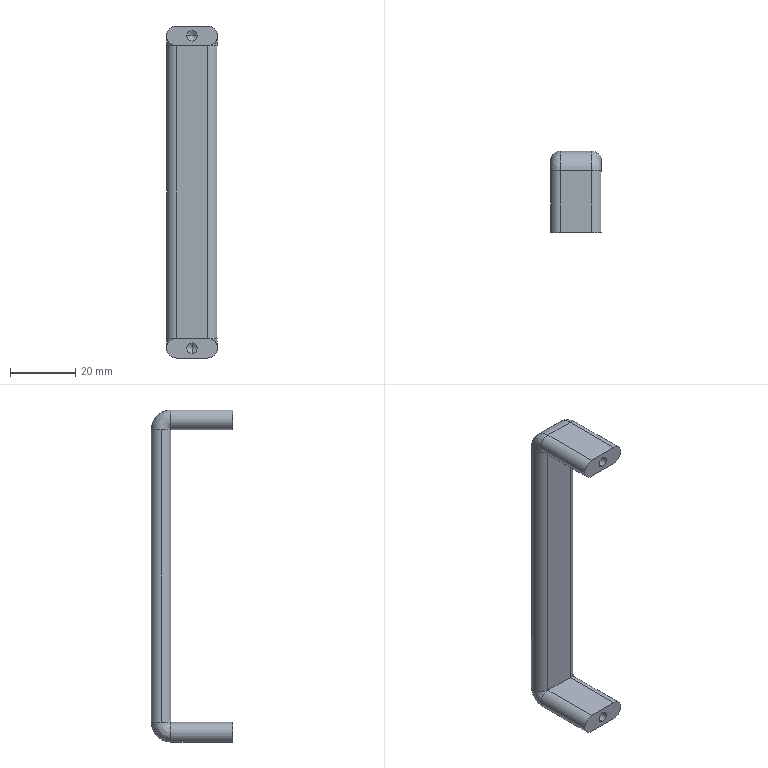Part | STEP file | AKM01-96 handle | 1 solid | 29 faces | box 15.6 x 25 x 102 mm | volume 11694 mm3 | cylinder 13 | plane 8 | cone 4 | spline 4 | commonest cylinder face diameters 6 x7 3.242 x4 12 x2
STEP:
#1=CARTESIAN_POINT('',(-4.8,19.,-6.));
#2=VERTEX_POINT('',#1);
#3=CARTESIAN_POINT('',(-7.8,22.,-6.));
#4=VERTEX_POINT('',#3);
#5=CARTESIAN_POINT('',(-4.8,22.,-6.));
#6=DIRECTION('',(0.,0.,-1.));
#7=DIRECTION('',(-1.,0.,0.));
#8=AXIS2_PLACEMENT_3D('',#5,#6,#7);
#9=CIRCLE('',#8,3.);
#10=EDGE_CURVE('',#2,#4,#9,.T.);
#11=ORIENTED_EDGE('',*,*,#10,.T.);
#12=CARTESIAN_POINT('',(-7.8,22.,-96.));
#13=VERTEX_POINT('',#12);
#14=CARTESIAN_POINT('',(-7.8,22.,-96.));
#15=DIRECTION('',(0.,0.,-1.));
#16=VECTOR('',#15,1000.);
#17=LINE('',#14,#16);
#18=EDGE_CURVE('',#4,#13,#17,.T.);
#19=ORIENTED_EDGE('',*,*,#18,.T.);
#20=CARTESIAN_POINT('',(-4.8,19.,-96.));
#21=VERTEX_POINT('',#20);
#22=CARTESIAN_POINT('',(-4.8,22.,-96.));
#23=DIRECTION('',(0.,0.,1.));
#24=DIRECTION('',(-1.,0.,0.));
#25=AXIS2_PLACEMENT_3D('',#22,#23,#24);
#26=CIRCLE('',#25,3.);
#27=EDGE_CURVE('',#13,#21,#26,.T.);
#28=ORIENTED_EDGE('',*,*,#27,.T.);
#29=CARTESIAN_POINT('',(-4.8,19.,-96.));
#30=DIRECTION('',(0.,0.,1.));
#31=VECTOR('',#30,1000.);
#32=LINE('',#29,#31);
#33=EDGE_CURVE('',#21,#2,#32,.T.);
#34=ORIENTED_EDGE('',*,*,#33,.T.);
#35=EDGE_LOOP('',(#11,#19,#28,#34));
#36=FACE_OUTER_BOUND('',#35,.T.);
#37=CARTESIAN_POINT('',(-4.8,22.,-96.));
#38=DIRECTION('',(0.,0.,-1.));
#39=DIRECTION('',(-1.,0.,0.));
#40=AXIS2_PLACEMENT_3D('',#37,#38,#39);
#41=CYLINDRICAL_SURFACE('',#40,3.);
#42=ADVANCED_FACE('',(#36),#41,.T.);
#43=CARTESIAN_POINT('',(0.,0.,-100.621));
#44=VERTEX_POINT('',#43);
#45=CARTESIAN_POINT('',(0.,0.,-97.379));
#46=VERTEX_POINT('',#45);
#47=CARTESIAN_POINT('',(0.,0.,-99.));
#48=DIRECTION('',(0.,1.,0.));
#49=DIRECTION('',(0.,0.,1.));
#50=AXIS2_PLACEMENT_3D('',#47,#48,#49);
#51=CIRCLE('',#50,1.621);
#52=EDGE_CURVE('',#44,#46,#51,.T.);
#53=ORIENTED_EDGE('',*,*,#52,.F.);
#54=CARTESIAN_POINT('',(0.,6.219,-100.621));
#55=VERTEX_POINT('',#54);
#56=CARTESIAN_POINT('',(0.,0.,-100.621));
#57=DIRECTION('',(0.,1.,0.));
#58=VECTOR('',#57,1000.);
#59=LINE('',#56,#58);
#60=EDGE_CURVE('',#44,#55,#59,.T.);
#61=ORIENTED_EDGE('',*,*,#60,.T.);
#62=CARTESIAN_POINT('',(0.,6.219,-97.379));
#63=VERTEX_POINT('',#62);
#64=CARTESIAN_POINT('',(0.,6.219,-99.));
#65=DIRECTION('',(0.,-1.,0.));
#66=DIRECTION('',(0.,0.,1.));
#67=AXIS2_PLACEMENT_3D('',#64,#65,#66);
#68=CIRCLE('',#67,1.621);
#69=EDGE_CURVE('',#63,#55,#68,.T.);
#70=ORIENTED_EDGE('',*,*,#69,.F.);
#71=CARTESIAN_POINT('',(0.,0.,-97.379));
#72=DIRECTION('',(0.,1.,0.));
#73=VECTOR('',#72,1000.);
#74=LINE('',#71,#73);
#75=EDGE_CURVE('',#46,#63,#74,.T.);
#76=ORIENTED_EDGE('',*,*,#75,.F.);
#77=EDGE_LOOP('',(#53,#61,#70,#76));
#78=FACE_OUTER_BOUND('',#77,.T.);
#79=CARTESIAN_POINT('',(0.,0.,-99.));
#80=DIRECTION('',(0.,1.,0.));
#81=DIRECTION('',(0.,0.,1.));
#82=AXIS2_PLACEMENT_3D('',#79,#80,#81);
#83=CYLINDRICAL_SURFACE('',#82,1.621);
#84=ADVANCED_FACE('',(#78),#83,.F.);
#85=CARTESIAN_POINT('',(0.,0.,-1.379));
#86=VERTEX_POINT('',#85);
#87=CARTESIAN_POINT('',(0.,0.,-4.621));
#88=VERTEX_POINT('',#87);
#89=CARTESIAN_POINT('',(0.,0.,-3.));
#90=DIRECTION('',(0.,-1.,0.));
#91=DIRECTION('',(0.,0.,1.));
#92=AXIS2_PLACEMENT_3D('',#89,#90,#91);
#93=CIRCLE('',#92,1.621);
#94=EDGE_CURVE('',#86,#88,#93,.T.);
#95=ORIENTED_EDGE('',*,*,#94,.T.);
#96=CARTESIAN_POINT('',(0.,6.219,-4.621));
#97=VERTEX_POINT('',#96);
#98=CARTESIAN_POINT('',(0.,0.,-4.621));
#99=DIRECTION('',(0.,1.,0.));
#100=VECTOR('',#99,1000.);
#101=LINE('',#98,#100);
#102=EDGE_CURVE('',#88,#97,#101,.T.);
#103=ORIENTED_EDGE('',*,*,#102,.T.);
#104=CARTESIAN_POINT('',(-1.621,6.219,-3.));
#105=VERTEX_POINT('',#104);
#106=CARTESIAN_POINT('',(0.,6.219,-3.));
#107=DIRECTION('',(0.,-1.,0.));
#108=DIRECTION('',(0.,0.,1.));
#109=AXIS2_PLACEMENT_3D('',#106,#107,#108);
#110=CIRCLE('',#109,1.621);
#111=EDGE_CURVE('',#105,#97,#110,.T.);
#112=ORIENTED_EDGE('',*,*,#111,.F.);
#113=CARTESIAN_POINT('',(0.,6.219,-1.379));
#114=VERTEX_POINT('',#113);
#115=CARTESIAN_POINT('',(0.,6.219,-3.));
#116=DIRECTION('',(0.,-1.,0.));
#117=DIRECTION('',(0.,0.,1.));
#118=AXIS2_PLACEMENT_3D('',#115,#116,#117);
#119=CIRCLE('',#118,1.621);
#120=EDGE_CURVE('',#114,#105,#119,.T.);
#121=ORIENTED_EDGE('',*,*,#120,.F.);
#122=CARTESIAN_POINT('',(0.,0.,-1.379));
#123=DIRECTION('',(0.,1.,0.));
#124=VECTOR('',#123,1000.);
#125=LINE('',#122,#124);
#126=EDGE_CURVE('',#86,#114,#125,.T.);
#127=ORIENTED_EDGE('',*,*,#126,.F.);
#128=EDGE_LOOP('',(#95,#103,#112,#121,#127));
#129=FACE_OUTER_BOUND('',#128,.T.);
#130=CARTESIAN_POINT('',(0.,0.,-3.));
#131=DIRECTION('',(0.,1.,0.));
#132=DIRECTION('',(0.,0.,1.));
#133=AXIS2_PLACEMENT_3D('',#130,#131,#132);
#134=CYLINDRICAL_SURFACE('',#133,1.621);
#135=ADVANCED_FACE('',(#129),#134,.F.);
#136=CARTESIAN_POINT('',(0.,7.155,-99.));
#137=VERTEX_POINT('',#136);
#138=CARTESIAN_POINT('',(0.,6.219,-100.621));
#139=DIRECTION('',(0.,-0.5,-0.866));
#140=VECTOR('',#139,1000.);
#141=LINE('',#138,#140);
#142=EDGE_CURVE('',#137,#55,#141,.T.);
#143=ORIENTED_EDGE('',*,*,#142,.F.);
#144=CARTESIAN_POINT('',(0.,6.219,-97.379));
#145=DIRECTION('',(0.,-0.5,0.866));
#146=VECTOR('',#145,1000.);
#147=LINE('',#144,#146);
#148=EDGE_CURVE('',#137,#63,#147,.T.);
#149=ORIENTED_EDGE('',*,*,#148,.T.);
#150=ORIENTED_EDGE('',*,*,#69,.T.);
#151=EDGE_LOOP('',(#143,#149,#150));
#152=FACE_OUTER_BOUND('',#151,.T.);
#153=CARTESIAN_POINT('',(0.,6.219,-99.));
#154=DIRECTION('',(0.,-1.,0.));
#155=DIRECTION('',(0.,0.,-1.));
#156=AXIS2_PLACEMENT_3D('',#153,#154,#155);
#157=CONICAL_SURFACE('',#156,1.621,1.047);
#158=ADVANCED_FACE('',(#152),#157,.F.);
#159=CARTESIAN_POINT('',(0.,7.155,-3.));
#160=VERTEX_POINT('',#159);
#161=CARTESIAN_POINT('',(1.621,6.219,-3.));
#162=VERTEX_POINT('',#161);
#163=CARTESIAN_POINT('',(1.621,6.219,-3.));
#164=DIRECTION('',(0.866,-0.5,0.));
#165=VECTOR('',#164,1000.);
#166=LINE('',#163,#165);
#167=EDGE_CURVE('',#160,#162,#166,.T.);
#168=ORIENTED_EDGE('',*,*,#167,.F.);
#169=CARTESIAN_POINT('',(-1.621,6.219,-3.));
#170=DIRECTION('',(-0.866,-0.5,0.));
#171=VECTOR('',#170,1000.);
#172=LINE('',#169,#171);
#173=EDGE_CURVE('',#160,#105,#172,.T.);
#174=ORIENTED_EDGE('',*,*,#173,.T.);
#175=ORIENTED_EDGE('',*,*,#111,.T.);
#176=CARTESIAN_POINT('',(0.,6.219,-3.));
#177=DIRECTION('',(0.,-1.,0.));
#178=DIRECTION('',(0.,0.,1.));
#179=AXIS2_PLACEMENT_3D('',#176,#177,#178);
#180=CIRCLE('',#179,1.621);
#181=EDGE_CURVE('',#97,#162,#180,.T.);
#182=ORIENTED_EDGE('',*,*,#181,.T.);
#183=EDGE_LOOP('',(#168,#174,#175,#182));
#184=FACE_OUTER_BOUND('',#183,.T.);
#185=CARTESIAN_POINT('',(0.,6.219,-3.));
#186=DIRECTION('',(0.,-1.,0.));
#187=DIRECTION('',(1.,0.,0.));
#188=AXIS2_PLACEMENT_3D('',#185,#186,#187);
#189=CONICAL_SURFACE('',#188,1.621,1.047);
#190=ADVANCED_FACE('',(#184),#189,.F.);
#191=CARTESIAN_POINT('',(4.8,19.,-6.));
#192=VERTEX_POINT('',#191);
#193=CARTESIAN_POINT('',(4.8,19.,-96.));
#194=VERTEX_POINT('',#193);
#195=CARTESIAN_POINT('',(4.8,19.,-96.));
#196=DIRECTION('',(0.,0.,-1.));
#197=VECTOR('',#196,1000.);
#198=LINE('',#195,#197);
#199=EDGE_CURVE('',#192,#194,#198,.T.);
#200=ORIENTED_EDGE('',*,*,#199,.F.);
#201=CARTESIAN_POINT('',(4.8,19.,-6.));
#202=DIRECTION('',(1.,0.,0.));
#203=VECTOR('',#202,1000.);
#204=LINE('',#201,#203);
#205=EDGE_CURVE('',#2,#192,#204,.T.);
#206=ORIENTED_EDGE('',*,*,#205,.F.);
#207=ORIENTED_EDGE('',*,*,#33,.F.);
#208=CARTESIAN_POINT('',(4.8,19.,-96.));
#209=DIRECTION('',(-1.,0.,0.));
#210=VECTOR('',#209,1000.);
#211=LINE('',#208,#210);
#212=EDGE_CURVE('',#194,#21,#211,.T.);
#213=ORIENTED_EDGE('',*,*,#212,.F.);
#214=EDGE_LOOP('',(#200,#206,#207,#213));
#215=FACE_OUTER_BOUND('',#214,.T.);
#216=CARTESIAN_POINT('',(4.8,19.,-96.));
#217=DIRECTION('',(0.,1.,0.));
#218=DIRECTION('',(0.,0.,1.));
#219=AXIS2_PLACEMENT_3D('',#216,#217,#218);
#220=PLANE('',#219);
#221=ADVANCED_FACE('',(#215),#220,.F.);
#222=CARTESIAN_POINT('',(-4.8,0.,-96.));
#223=VERTEX_POINT('',#222);
#224=CARTESIAN_POINT('',(-4.8,0.,-96.));
#225=DIRECTION('',(0.,1.,0.));
#226=VECTOR('',#225,1000.);
#227=LINE('',#224,#226);
#228=EDGE_CURVE('',#223,#21,#227,.T.);
#229=ORIENTED_EDGE('',*,*,#228,.F.);
#230=CARTESIAN_POINT('',(4.8,0.,-96.));
#231=VERTEX_POINT('',#230);
#232=CARTESIAN_POINT('',(4.8,0.,-96.));
#233=DIRECTION('',(-1.,0.,0.));
#234=VECTOR('',#233,1000.);
#235=LINE('',#232,#234);
#236=EDGE_CURVE('',#231,#223,#235,.T.);
#237=ORIENTED_EDGE('',*,*,#236,.F.);
#238=CARTESIAN_POINT('',(4.8,0.,-96.));
#239=DIRECTION('',(0.,-1.,0.));
#240=VECTOR('',#239,1000.);
#241=LINE('',#238,#240);
#242=EDGE_CURVE('',#194,#231,#241,.T.);
#243=ORIENTED_EDGE('',*,*,#242,.F.);
#244=ORIENTED_EDGE('',*,*,#212,.T.);
#245=EDGE_LOOP('',(#229,#237,#243,#244));
#246=FACE_OUTER_BOUND('',#245,.T.);
#247=CARTESIAN_POINT('',(4.8,0.,-96.));
#248=DIRECTION('',(0.,0.,-1.));
#249=DIRECTION('',(-1.,0.,0.));
#250=AXIS2_PLACEMENT_3D('',#247,#248,#249);
#251=PLANE('',#250);
#252=ADVANCED_FACE('',(#246),#251,.F.);
#253=CARTESIAN_POINT('',(4.8,25.,-96.));
#254=VERTEX_POINT('',#253);
#255=CARTESIAN_POINT('',(4.8,22.,-96.));
#256=DIRECTION('',(0.,0.,1.));
#257=DIRECTION('',(-1.,0.,0.));
#258=AXIS2_PLACEMENT_3D('',#255,#256,#257);
#259=CIRCLE('',#258,3.);
#260=EDGE_CURVE('',#194,#254,#259,.T.);
#261=ORIENTED_EDGE('',*,*,#260,.T.);
#262=CARTESIAN_POINT('',(4.8,25.,-6.));
#263=VERTEX_POINT('',#262);
#264=CARTESIAN_POINT('',(4.8,25.,-96.));
#265=DIRECTION('',(0.,0.,1.));
#266=VECTOR('',#265,1000.);
#267=LINE('',#264,#266);
#268=EDGE_CURVE('',#254,#263,#267,.T.);
#269=ORIENTED_EDGE('',*,*,#268,.T.);
#270=CARTESIAN_POINT('',(4.8,22.,-6.));
#271=DIRECTION('',(0.,0.,-1.));
#272=DIRECTION('',(-1.,0.,0.));
#273=AXIS2_PLACEMENT_3D('',#270,#271,#272);
#274=CIRCLE('',#273,3.);
#275=EDGE_CURVE('',#263,#192,#274,.T.);
#276=ORIENTED_EDGE('',*,*,#275,.T.);
#277=ORIENTED_EDGE('',*,*,#199,.T.);
#278=EDGE_LOOP('',(#261,#269,#276,#277));
#279=FACE_OUTER_BOUND('',#278,.T.);
#280=CARTESIAN_POINT('',(4.8,22.,-96.));
#281=DIRECTION('',(0.,0.,-1.));
#282=DIRECTION('',(-1.,0.,0.));
#283=AXIS2_PLACEMENT_3D('',#280,#281,#282);
#284=CYLINDRICAL_SURFACE('',#283,3.);
#285=ADVANCED_FACE('',(#279),#284,.T.);
#286=CARTESIAN_POINT('',(4.8,0.,-6.));
#287=VERTEX_POINT('',#286);
#288=CARTESIAN_POINT('',(4.8,19.,-6.));
#289=DIRECTION('',(0.,1.,0.));
#290=VECTOR('',#289,1000.);
#291=LINE('',#288,#290);
#292=EDGE_CURVE('',#287,#192,#291,.T.);
#293=ORIENTED_EDGE('',*,*,#292,.F.);
#294=CARTESIAN_POINT('',(-4.8,0.,-6.));
#295=VERTEX_POINT('',#294);
#296=CARTESIAN_POINT('',(4.8,0.,-6.));
#297=DIRECTION('',(1.,0.,0.));
#298=VECTOR('',#297,1000.);
#299=LINE('',#296,#298);
#300=EDGE_CURVE('',#295,#287,#299,.T.);
#301=ORIENTED_EDGE('',*,*,#300,.F.);
#302=CARTESIAN_POINT('',(-4.8,19.,-6.));
#303=DIRECTION('',(0.,-1.,0.));
#304=VECTOR('',#303,1000.);
#305=LINE('',#302,#304);
#306=EDGE_CURVE('',#2,#295,#305,.T.);
#307=ORIENTED_EDGE('',*,*,#306,.F.);
#308=ORIENTED_EDGE('',*,*,#205,.T.);
#309=EDGE_LOOP('',(#293,#301,#307,#308));
#310=FACE_OUTER_BOUND('',#309,.T.);
#311=CARTESIAN_POINT('',(4.8,19.,-6.));
#312=DIRECTION('',(0.,0.,1.));
#313=DIRECTION('',(1.,0.,0.));
#314=AXIS2_PLACEMENT_3D('',#311,#312,#313);
#315=PLANE('',#314);
#316=ADVANCED_FACE('',(#310),#315,.F.);
#317=ORIENTED_EDGE('',*,*,#18,.F.);
#318=CARTESIAN_POINT('',(-4.8,25.,-6.));
#319=VERTEX_POINT('',#318);
#320=CARTESIAN_POINT('',(-4.8,22.,-6.));
#321=DIRECTION('',(0.,0.,-1.));
#322=DIRECTION('',(-1.,0.,0.));
#323=AXIS2_PLACEMENT_3D('',#320,#321,#322);
#324=CIRCLE('',#323,3.);
#325=EDGE_CURVE('',#4,#319,#324,.T.);
#326=ORIENTED_EDGE('',*,*,#325,.T.);
#327=CARTESIAN_POINT('',(-4.8,25.,-96.));
#328=VERTEX_POINT('',#327);
#329=CARTESIAN_POINT('',(-4.8,25.,-96.));
#330=DIRECTION('',(0.,0.,-1.));
#331=VECTOR('',#330,1000.);
#332=LINE('',#329,#331);
#333=EDGE_CURVE('',#319,#328,#332,.T.);
#334=ORIENTED_EDGE('',*,*,#333,.T.);
#335=CARTESIAN_POINT('',(-4.8,22.,-96.));
#336=DIRECTION('',(0.,0.,1.));
#337=DIRECTION('',(-1.,0.,0.));
#338=AXIS2_PLACEMENT_3D('',#335,#336,#337);
#339=CIRCLE('',#338,3.);
#340=EDGE_CURVE('',#328,#13,#339,.T.);
#341=ORIENTED_EDGE('',*,*,#340,.T.);
#342=EDGE_LOOP('',(#317,#326,#334,#341));
#343=FACE_OUTER_BOUND('',#342,.T.);
#344=CARTESIAN_POINT('',(-4.8,22.,-96.));
#345=DIRECTION('',(0.,0.,-1.));
#346=DIRECTION('',(-1.,0.,0.));
#347=AXIS2_PLACEMENT_3D('',#344,#345,#346);
#348=CYLINDRICAL_SURFACE('',#347,3.);
#349=ADVANCED_FACE('',(#343),#348,.T.);
#350=CARTESIAN_POINT('',(-4.8,0.,-102.));
#351=VERTEX_POINT('',#350);
#352=CARTESIAN_POINT('',(-4.8,0.,-99.));
#353=DIRECTION('',(0.,1.,0.));
#354=DIRECTION('',(0.,0.,-1.));
#355=AXIS2_PLACEMENT_3D('',#352,#353,#354);
#356=CIRCLE('',#355,3.);
#357=EDGE_CURVE('',#351,#223,#356,.T.);
#358=ORIENTED_EDGE('',*,*,#357,.T.);
#359=ORIENTED_EDGE('',*,*,#228,.T.);
#360=CARTESIAN_POINT('',(-4.8,19.,-102.));
#361=VERTEX_POINT('',#360);
#362=CARTESIAN_POINT('',(-4.8,19.,-99.));
#363=DIRECTION('',(0.,-1.,0.));
#364=DIRECTION('',(0.,0.,-1.));
#365=AXIS2_PLACEMENT_3D('',#362,#363,#364);
#366=CIRCLE('',#365,3.);
#367=EDGE_CURVE('',#21,#361,#366,.T.);
#368=ORIENTED_EDGE('',*,*,#367,.T.);
#369=CARTESIAN_POINT('',(-4.8,0.,-102.));
#370=DIRECTION('',(0.,-1.,0.));
#371=VECTOR('',#370,1000.);
#372=LINE('',#369,#371);
#373=EDGE_CURVE('',#361,#351,#372,.T.);
#374=ORIENTED_EDGE('',*,*,#373,.T.);
#375=EDGE_LOOP('',(#358,#359,#368,#374));
#376=FACE_OUTER_BOUND('',#375,.T.);
#377=CARTESIAN_POINT('',(-4.8,0.,-99.));
#378=DIRECTION('',(0.,-1.,0.));
#379=DIRECTION('',(0.,0.,-1.));
#380=AXIS2_PLACEMENT_3D('',#377,#378,#379);
#381=CYLINDRICAL_SURFACE('',#380,3.);
#382=ADVANCED_FACE('',(#376),#381,.T.);
#383=CARTESIAN_POINT('',(4.8,0.,-102.));
#384=VERTEX_POINT('',#383);
#385=CARTESIAN_POINT('',(-4.8,0.,-102.));
#386=DIRECTION('',(1.,0.,0.));
#387=VECTOR('',#386,1000.);
#388=LINE('',#385,#387);
#389=EDGE_CURVE('',#351,#384,#388,.T.);
#390=ORIENTED_EDGE('',*,*,#389,.T.);
#391=CARTESIAN_POINT('',(4.8,0.,-99.));
#392=DIRECTION('',(0.,-1.,0.));
#393=DIRECTION('',(0.,0.,-1.));
#394=AXIS2_PLACEMENT_3D('',#391,#392,#393);
#395=CIRCLE('',#394,3.);
#396=EDGE_CURVE('',#384,#231,#395,.T.);
#397=ORIENTED_EDGE('',*,*,#396,.T.);
#398=ORIENTED_EDGE('',*,*,#236,.T.);
#399=ORIENTED_EDGE('',*,*,#357,.F.);
#400=EDGE_LOOP('',(#390,#397,#398,#399));
#401=FACE_OUTER_BOUND('',#400,.T.);
#402=CARTESIAN_POINT('',(0.,0.,-99.));
#403=DIRECTION('',(0.,1.,0.));
#404=DIRECTION('',(0.,0.,1.));
#405=AXIS2_PLACEMENT_3D('',#402,#403,#404);
#406=CIRCLE('',#405,1.621);
#407=EDGE_CURVE('',#46,#44,#406,.T.);
#408=ORIENTED_EDGE('',*,*,#407,.T.);
#409=ORIENTED_EDGE('',*,*,#52,.T.);
#410=EDGE_LOOP('',(#408,#409));
#411=FACE_BOUND('',#410,.T.);
#412=CARTESIAN_POINT('',(-4.8,0.,-99.));
#413=DIRECTION('',(0.,-1.,0.));
#414=DIRECTION('',(0.,0.,-1.));
#415=AXIS2_PLACEMENT_3D('',#412,#413,#414);
#416=PLANE('',#415);
#417=ADVANCED_FACE('',(#401,#411),#416,.T.);
#418=ORIENTED_EDGE('',*,*,#396,.F.);
#419=CARTESIAN_POINT('',(4.8,19.,-102.));
#420=VERTEX_POINT('',#419);
#421=CARTESIAN_POINT('',(4.8,0.,-102.));
#422=DIRECTION('',(0.,1.,0.));
#423=VECTOR('',#422,1000.);
#424=LINE('',#421,#423);
#425=EDGE_CURVE('',#384,#420,#424,.T.);
#426=ORIENTED_EDGE('',*,*,#425,.T.);
#427=CARTESIAN_POINT('',(4.8,19.,-99.));
#428=DIRECTION('',(0.,-1.,0.));
#429=DIRECTION('',(0.,0.,-1.));
#430=AXIS2_PLACEMENT_3D('',#427,#428,#429);
#431=CIRCLE('',#430,3.);
#432=EDGE_CURVE('',#420,#194,#431,.T.);
#433=ORIENTED_EDGE('',*,*,#432,.T.);
#434=ORIENTED_EDGE('',*,*,#242,.T.);
#435=EDGE_LOOP('',(#418,#426,#433,#434));
#436=FACE_OUTER_BOUND('',#435,.T.);
#437=CARTESIAN_POINT('',(4.8,0.,-99.));
#438=DIRECTION('',(0.,-1.,0.));
#439=DIRECTION('',(0.,0.,-1.));
#440=AXIS2_PLACEMENT_3D('',#437,#438,#439);
#441=CYLINDRICAL_SURFACE('',#440,3.);
#442=ADVANCED_FACE('',(#436),#441,.T.);
#443=ORIENTED_EDGE('',*,*,#268,.F.);
#444=CARTESIAN_POINT('',(-4.8,25.,-96.));
#445=DIRECTION('',(1.,0.,0.));
#446=VECTOR('',#445,1000.);
#447=LINE('',#444,#446);
#448=EDGE_CURVE('',#328,#254,#447,.T.);
#449=ORIENTED_EDGE('',*,*,#448,.F.);
#450=ORIENTED_EDGE('',*,*,#333,.F.);
#451=CARTESIAN_POINT('',(-4.8,25.,-6.));
#452=DIRECTION('',(-1.,0.,0.));
#453=VECTOR('',#452,1000.);
#454=LINE('',#451,#453);
#455=EDGE_CURVE('',#263,#319,#454,.T.);
#456=ORIENTED_EDGE('',*,*,#455,.F.);
#457=EDGE_LOOP('',(#443,#449,#450,#456));
#458=FACE_OUTER_BOUND('',#457,.T.);
#459=CARTESIAN_POINT('',(-4.8,25.,-96.));
#460=DIRECTION('',(0.,-1.,0.));
#461=DIRECTION('',(0.,0.,-1.));
#462=AXIS2_PLACEMENT_3D('',#459,#460,#461);
#463=PLANE('',#462);
#464=ADVANCED_FACE('',(#458),#463,.F.);
#465=ORIENTED_EDGE('',*,*,#260,.F.);
#466=ORIENTED_EDGE('',*,*,#432,.F.);
#467=CARTESIAN_POINT('',(4.8,19.,-96.));
#468=DIRECTION('',(1.,0.,0.));
#469=DIRECTION('',(0.,0.,1.));
#470=AXIS2_PLACEMENT_3D('',#467,#468,#469);
#471=CIRCLE('',#470,6.);
#472=EDGE_CURVE('',#420,#254,#471,.T.);
#473=ORIENTED_EDGE('',*,*,#472,.T.);
#474=EDGE_LOOP('',(#465,#466,#473));
#475=FACE_OUTER_BOUND('',#474,.T.);
#476=CARTESIAN_POINT('',(4.8,25.,-96.));
#477=CARTESIAN_POINT('',(4.8,25.,-99.515));
#478=CARTESIAN_POINT('',(4.8,22.515,-102.));
#479=CARTESIAN_POINT('',(4.8,19.,-102.));
#480=CARTESIAN_POINT('',(10.8,25.,-96.));
#481=CARTESIAN_POINT('',(10.8,25.,-99.515));
#482=CARTESIAN_POINT('',(10.8,22.515,-102.));
#483=CARTESIAN_POINT('',(10.8,19.,-102.));
#484=CARTESIAN_POINT('',(10.8,19.,-96.));
#485=CARTESIAN_POINT('',(10.8,19.,-96.));
#486=CARTESIAN_POINT('',(10.8,19.,-96.));
#487=CARTESIAN_POINT('',(10.8,19.,-96.));
#488=CARTESIAN_POINT('',(4.8,19.,-96.));
#489=CARTESIAN_POINT('',(4.8,19.,-96.));
#490=CARTESIAN_POINT('',(4.8,19.,-96.));
#491=CARTESIAN_POINT('',(4.8,19.,-96.));
#492=(BOUNDED_SURFACE()B_SPLINE_SURFACE(3,3,((#476,#477,#478,#479),(#480,#481,#482,#483),(#484,#485,#486,#487),(#488,#489,#490,#491)),.UNSPECIFIED.,.F.,.F.,.F.)B_SPLINE_SURFACE_WITH_KNOTS((4,4),(4,4),(0.,1.),(0.,1.),.UNSPECIFIED.)GEOMETRIC_REPRESENTATION_ITEM()RATIONAL_B_SPLINE_SURFACE(((1.,0.8047,0.8047,1.),(0.3333,0.2682,0.2682,0.3333),(0.3333,0.2682,0.2682,0.3333),(1.,0.8047,0.8047,1.)))REPRESENTATION_ITEM('')SURFACE());
#493=ADVANCED_FACE('',(#475),#492,.T.);
#494=CARTESIAN_POINT('',(4.8,19.,0.));
#495=VERTEX_POINT('',#494);
#496=CARTESIAN_POINT('',(4.8,19.,-3.));
#497=DIRECTION('',(0.,1.,0.));
#498=DIRECTION('',(0.,0.,1.));
#499=AXIS2_PLACEMENT_3D('',#496,#497,#498);
#500=CIRCLE('',#499,3.);
#501=EDGE_CURVE('',#495,#192,#500,.T.);
#502=ORIENTED_EDGE('',*,*,#501,.T.);
#503=ORIENTED_EDGE('',*,*,#275,.F.);
#504=CARTESIAN_POINT('',(4.8,19.,-6.));
#505=DIRECTION('',(1.,0.,0.));
#506=DIRECTION('',(0.,0.,1.));
#507=AXIS2_PLACEMENT_3D('',#504,#505,#506);
#508=CIRCLE('',#507,6.);
#509=EDGE_CURVE('',#263,#495,#508,.T.);
#510=ORIENTED_EDGE('',*,*,#509,.T.);
#511=EDGE_LOOP('',(#502,#503,#510));
#512=FACE_OUTER_BOUND('',#511,.T.);
#513=CARTESIAN_POINT('',(4.8,19.,0.));
#514=CARTESIAN_POINT('',(4.8,22.515,0.));
#515=CARTESIAN_POINT('',(4.8,25.,-2.485));
#516=CARTESIAN_POINT('',(4.8,25.,-6.));
#517=CARTESIAN_POINT('',(10.8,19.,0.));
#518=CARTESIAN_POINT('',(10.8,22.515,0.));
#519=CARTESIAN_POINT('',(10.8,25.,-2.485));
#520=CARTESIAN_POINT('',(10.8,25.,-6.));
#521=CARTESIAN_POINT('',(10.8,19.,-6.));
#522=CARTESIAN_POINT('',(10.8,19.,-6.));
#523=CARTESIAN_POINT('',(10.8,19.,-6.));
#524=CARTESIAN_POINT('',(10.8,19.,-6.));
#525=CARTESIAN_POINT('',(4.8,19.,-6.));
#526=CARTESIAN_POINT('',(4.8,19.,-6.));
#527=CARTESIAN_POINT('',(4.8,19.,-6.));
#528=CARTESIAN_POINT('',(4.8,19.,-6.));
#529=(BOUNDED_SURFACE()B_SPLINE_SURFACE(3,3,((#513,#514,#515,#516),(#517,#518,#519,#520),(#521,#522,#523,#524),(#525,#526,#527,#528)),.UNSPECIFIED.,.F.,.F.,.F.)B_SPLINE_SURFACE_WITH_KNOTS((4,4),(4,4),(0.,1.),(0.,1.),.UNSPECIFIED.)GEOMETRIC_REPRESENTATION_ITEM()RATIONAL_B_SPLINE_SURFACE(((1.,0.8047,0.8047,1.),(0.3333,0.2682,0.2682,0.3333),(0.3333,0.2682,0.2682,0.3333),(1.,0.8047,0.8047,1.)))REPRESENTATION_ITEM('')SURFACE());
#530=ADVANCED_FACE('',(#512),#529,.T.);
#531=ORIENTED_EDGE('',*,*,#501,.F.);
#532=CARTESIAN_POINT('',(4.8,0.,0.));
#533=VERTEX_POINT('',#532);
#534=CARTESIAN_POINT('',(4.8,19.,0.));
#535=DIRECTION('',(0.,-1.,0.));
#536=VECTOR('',#535,1000.);
#537=LINE('',#534,#536);
#538=EDGE_CURVE('',#495,#533,#537,.T.);
#539=ORIENTED_EDGE('',*,*,#538,.T.);
#540=CARTESIAN_POINT('',(4.8,0.,-3.));
#541=DIRECTION('',(0.,1.,0.));
#542=DIRECTION('',(0.,0.,1.));
#543=AXIS2_PLACEMENT_3D('',#540,#541,#542);
#544=CIRCLE('',#543,3.);
#545=EDGE_CURVE('',#533,#287,#544,.T.);
#546=ORIENTED_EDGE('',*,*,#545,.T.);
#547=ORIENTED_EDGE('',*,*,#292,.T.);
#548=EDGE_LOOP('',(#531,#539,#546,#547));
#549=FACE_OUTER_BOUND('',#548,.T.);
#550=CARTESIAN_POINT('',(4.8,19.,-3.));
#551=DIRECTION('',(0.,1.,0.));
#552=DIRECTION('',(0.,0.,1.));
#553=AXIS2_PLACEMENT_3D('',#550,#551,#552);
#554=CYLINDRICAL_SURFACE('',#553,3.);
#555=ADVANCED_FACE('',(#549),#554,.T.);
#556=ORIENTED_EDGE('',*,*,#545,.F.);
#557=CARTESIAN_POINT('',(-4.8,0.,0.));
#558=VERTEX_POINT('',#557);
#559=CARTESIAN_POINT('',(-4.8,0.,0.));
#560=DIRECTION('',(1.,0.,0.));
#561=VECTOR('',#560,1000.);
#562=LINE('',#559,#561);
#563=EDGE_CURVE('',#558,#533,#562,.T.);
#564=ORIENTED_EDGE('',*,*,#563,.F.);
#565=CARTESIAN_POINT('',(-4.8,0.,-3.));
#566=DIRECTION('',(0.,1.,0.));
#567=DIRECTION('',(0.,0.,1.));
#568=AXIS2_PLACEMENT_3D('',#565,#566,#567);
#569=CIRCLE('',#568,3.);
#570=EDGE_CURVE('',#295,#558,#569,.T.);
#571=ORIENTED_EDGE('',*,*,#570,.F.);
#572=ORIENTED_EDGE('',*,*,#300,.T.);
#573=EDGE_LOOP('',(#556,#564,#571,#572));
#574=FACE_OUTER_BOUND('',#573,.T.);
#575=ORIENTED_EDGE('',*,*,#94,.F.);
#576=CARTESIAN_POINT('',(0.,0.,-3.));
#577=DIRECTION('',(0.,-1.,0.));
#578=DIRECTION('',(0.,0.,1.));
#579=AXIS2_PLACEMENT_3D('',#576,#577,#578);
#580=CIRCLE('',#579,1.621);
#581=EDGE_CURVE('',#88,#86,#580,.T.);
#582=ORIENTED_EDGE('',*,*,#581,.F.);
#583=EDGE_LOOP('',(#575,#582));
#584=FACE_BOUND('',#583,.T.);
#585=CARTESIAN_POINT('',(-4.8,0.,-3.));
#586=DIRECTION('',(0.,1.,0.));
#587=DIRECTION('',(0.,0.,1.));
#588=AXIS2_PLACEMENT_3D('',#585,#586,#587);
#589=PLANE('',#588);
#590=ADVANCED_FACE('',(#574,#584),#589,.F.);
#591=CARTESIAN_POINT('',(-4.8,19.,0.));
#592=VERTEX_POINT('',#591);
#593=CARTESIAN_POINT('',(-4.8,19.,-3.));
#594=DIRECTION('',(0.,-1.,0.));
#595=DIRECTION('',(0.,0.,1.));
#596=AXIS2_PLACEMENT_3D('',#593,#594,#595);
#597=CIRCLE('',#596,3.);
#598=EDGE_CURVE('',#592,#2,#597,.T.);
#599=ORIENTED_EDGE('',*,*,#598,.T.);
#600=ORIENTED_EDGE('',*,*,#306,.T.);
#601=ORIENTED_EDGE('',*,*,#570,.T.);
#602=CARTESIAN_POINT('',(-4.8,19.,0.));
#603=DIRECTION('',(0.,1.,0.));
#604=VECTOR('',#603,1000.);
#605=LINE('',#602,#604);
#606=EDGE_CURVE('',#558,#592,#605,.T.);
#607=ORIENTED_EDGE('',*,*,#606,.T.);
#608=EDGE_LOOP('',(#599,#600,#601,#607));
#609=FACE_OUTER_BOUND('',#608,.T.);
#610=CARTESIAN_POINT('',(-4.8,19.,-3.));
#611=DIRECTION('',(0.,1.,0.));
#612=DIRECTION('',(0.,0.,1.));
#613=AXIS2_PLACEMENT_3D('',#610,#611,#612);
#614=CYLINDRICAL_SURFACE('',#613,3.);
#615=ADVANCED_FACE('',(#609),#614,.T.);
#616=CARTESIAN_POINT('',(-4.8,19.,-96.));
#617=DIRECTION('',(-1.,0.,0.));
#618=DIRECTION('',(0.,0.,1.));
#619=AXIS2_PLACEMENT_3D('',#616,#617,#618);
#620=CIRCLE('',#619,6.);
#621=EDGE_CURVE('',#328,#361,#620,.T.);
#622=ORIENTED_EDGE('',*,*,#621,.T.);
#623=ORIENTED_EDGE('',*,*,#367,.F.);
#624=ORIENTED_EDGE('',*,*,#27,.F.);
#625=ORIENTED_EDGE('',*,*,#340,.F.);
#626=EDGE_LOOP('',(#622,#623,#624,#625));
#627=FACE_OUTER_BOUND('',#626,.T.);
#628=CARTESIAN_POINT('',(-4.8,19.,-96.));
#629=CARTESIAN_POINT('',(-4.8,19.,-96.));
#630=CARTESIAN_POINT('',(-4.8,19.,-96.));
#631=CARTESIAN_POINT('',(-4.8,19.,-96.));
#632=CARTESIAN_POINT('',(-4.8,19.,-96.));
#633=CARTESIAN_POINT('',(-4.8,19.,-96.));
#634=CARTESIAN_POINT('',(-4.8,19.,-96.));
#635=CARTESIAN_POINT('',(-10.8,19.,-96.));
#636=CARTESIAN_POINT('',(-10.8,19.,-96.));
#637=CARTESIAN_POINT('',(-10.8,19.,-96.));
#638=CARTESIAN_POINT('',(-10.8,19.,-96.));
#639=CARTESIAN_POINT('',(-10.8,19.,-96.));
#640=CARTESIAN_POINT('',(-10.8,19.,-96.));
#641=CARTESIAN_POINT('',(-10.8,19.,-96.));
#642=CARTESIAN_POINT('',(-10.8,19.,-90.));
#643=CARTESIAN_POINT('',(-10.8,31.,-90.));
#644=CARTESIAN_POINT('',(-10.8,31.,-102.));
#645=CARTESIAN_POINT('',(-10.8,19.,-102.));
#646=CARTESIAN_POINT('',(-10.8,7.,-102.));
#647=CARTESIAN_POINT('',(-10.8,7.,-90.));
#648=CARTESIAN_POINT('',(-10.8,19.,-90.));
#649=CARTESIAN_POINT('',(-4.8,19.,-90.));
#650=CARTESIAN_POINT('',(-4.8,31.,-90.));
#651=CARTESIAN_POINT('',(-4.8,31.,-102.));
#652=CARTESIAN_POINT('',(-4.8,19.,-102.));
#653=CARTESIAN_POINT('',(-4.8,7.,-102.));
#654=CARTESIAN_POINT('',(-4.8,7.,-90.));
#655=CARTESIAN_POINT('',(-4.8,19.,-90.));
#656=CARTESIAN_POINT('',(1.2,19.,-90.));
#657=CARTESIAN_POINT('',(1.2,31.,-90.));
#658=CARTESIAN_POINT('',(1.2,31.,-102.));
#659=CARTESIAN_POINT('',(1.2,19.,-102.));
#660=CARTESIAN_POINT('',(1.2,7.,-102.));
#661=CARTESIAN_POINT('',(1.2,7.,-90.));
#662=CARTESIAN_POINT('',(1.2,19.,-90.));
#663=CARTESIAN_POINT('',(1.2,19.,-96.));
#664=CARTESIAN_POINT('',(1.2,19.,-96.));
#665=CARTESIAN_POINT('',(1.2,19.,-96.));
#666=CARTESIAN_POINT('',(1.2,19.,-96.));
#667=CARTESIAN_POINT('',(1.2,19.,-96.));
#668=CARTESIAN_POINT('',(1.2,19.,-96.));
#669=CARTESIAN_POINT('',(1.2,19.,-96.));
#670=CARTESIAN_POINT('',(-4.8,19.,-96.));
#671=CARTESIAN_POINT('',(-4.8,19.,-96.));
#672=CARTESIAN_POINT('',(-4.8,19.,-96.));
#673=CARTESIAN_POINT('',(-4.8,19.,-96.));
#674=CARTESIAN_POINT('',(-4.8,19.,-96.));
#675=CARTESIAN_POINT('',(-4.8,19.,-96.));
#676=CARTESIAN_POINT('',(-4.8,19.,-96.));
#677=(BOUNDED_SURFACE()B_SPLINE_SURFACE(3,3,((#628,#629,#630,#631,#632,#633,#634),(#635,#636,#637,#638,#639,#640,#641),(#642,#643,#644,#645,#646,#647,#648),(#649,#650,#651,#652,#653,#654,#655),(#656,#657,#658,#659,#660,#661,#662),(#663,#664,#665,#666,#667,#668,#669),(#670,#671,#672,#673,#674,#675,#676)),.UNSPECIFIED.,.T.,.T.,.F.)B_SPLINE_SURFACE_WITH_KNOTS((4,3,4),(4,3,4),(0.,0.5,1.),(0.,0.5,1.),.UNSPECIFIED.)GEOMETRIC_REPRESENTATION_ITEM()RATIONAL_B_SPLINE_SURFACE(((1.,0.3333,0.3333,1.,0.3333,0.3333,1.),(0.3333,0.1111,0.1111,0.3333,0.1111,0.1111,0.3333),(0.3333,0.1111,0.1111,0.3333,0.1111,0.1111,0.3333),(1.,0.3333,0.3333,1.,0.3333,0.3333,1.),(0.3333,0.1111,0.1111,0.3333,0.1111,0.1111,0.3333),(0.3333,0.1111,0.1111,0.3333,0.1111,0.1111,0.3333),(1.,0.3333,0.3333,1.,0.3333,0.3333,1.)))REPRESENTATION_ITEM('')SURFACE());
#678=ADVANCED_FACE('',(#627),#677,.T.);
#679=CARTESIAN_POINT('',(-4.8,19.,-6.));
#680=DIRECTION('',(-1.,0.,0.));
#681=DIRECTION('',(0.,0.,1.));
#682=AXIS2_PLACEMENT_3D('',#679,#680,#681);
#683=CIRCLE('',#682,6.);
#684=EDGE_CURVE('',#592,#319,#683,.T.);
#685=ORIENTED_EDGE('',*,*,#684,.T.);
#686=ORIENTED_EDGE('',*,*,#325,.F.);
#687=ORIENTED_EDGE('',*,*,#10,.F.);
#688=ORIENTED_EDGE('',*,*,#598,.F.);
#689=EDGE_LOOP('',(#685,#686,#687,#688));
#690=FACE_OUTER_BOUND('',#689,.T.);
#691=CARTESIAN_POINT('',(-4.8,19.,-6.));
#692=CARTESIAN_POINT('',(-4.8,19.,-6.));
#693=CARTESIAN_POINT('',(-4.8,19.,-6.));
#694=CARTESIAN_POINT('',(-4.8,19.,-6.));
#695=CARTESIAN_POINT('',(-4.8,19.,-6.));
#696=CARTESIAN_POINT('',(-4.8,19.,-6.));
#697=CARTESIAN_POINT('',(-4.8,19.,-6.));
#698=CARTESIAN_POINT('',(-10.8,19.,-6.));
#699=CARTESIAN_POINT('',(-10.8,19.,-6.));
#700=CARTESIAN_POINT('',(-10.8,19.,-6.));
#701=CARTESIAN_POINT('',(-10.8,19.,-6.));
#702=CARTESIAN_POINT('',(-10.8,19.,-6.));
#703=CARTESIAN_POINT('',(-10.8,19.,-6.));
#704=CARTESIAN_POINT('',(-10.8,19.,-6.));
#705=CARTESIAN_POINT('',(-10.8,19.,0.));
#706=CARTESIAN_POINT('',(-10.8,31.,0.));
#707=CARTESIAN_POINT('',(-10.8,31.,-12.));
#708=CARTESIAN_POINT('',(-10.8,19.,-12.));
#709=CARTESIAN_POINT('',(-10.8,7.,-12.));
#710=CARTESIAN_POINT('',(-10.8,7.,0.));
#711=CARTESIAN_POINT('',(-10.8,19.,0.));
#712=CARTESIAN_POINT('',(-4.8,19.,0.));
#713=CARTESIAN_POINT('',(-4.8,31.,0.));
#714=CARTESIAN_POINT('',(-4.8,31.,-12.));
#715=CARTESIAN_POINT('',(-4.8,19.,-12.));
#716=CARTESIAN_POINT('',(-4.8,7.,-12.));
#717=CARTESIAN_POINT('',(-4.8,7.,0.));
#718=CARTESIAN_POINT('',(-4.8,19.,0.));
#719=CARTESIAN_POINT('',(1.2,19.,0.));
#720=CARTESIAN_POINT('',(1.2,31.,0.));
#721=CARTESIAN_POINT('',(1.2,31.,-12.));
#722=CARTESIAN_POINT('',(1.2,19.,-12.));
#723=CARTESIAN_POINT('',(1.2,7.,-12.));
#724=CARTESIAN_POINT('',(1.2,7.,0.));
#725=CARTESIAN_POINT('',(1.2,19.,0.));
#726=CARTESIAN_POINT('',(1.2,19.,-6.));
#727=CARTESIAN_POINT('',(1.2,19.,-6.));
#728=CARTESIAN_POINT('',(1.2,19.,-6.));
#729=CARTESIAN_POINT('',(1.2,19.,-6.));
#730=CARTESIAN_POINT('',(1.2,19.,-6.));
#731=CARTESIAN_POINT('',(1.2,19.,-6.));
#732=CARTESIAN_POINT('',(1.2,19.,-6.));
#733=CARTESIAN_POINT('',(-4.8,19.,-6.));
#734=CARTESIAN_POINT('',(-4.8,19.,-6.));
#735=CARTESIAN_POINT('',(-4.8,19.,-6.));
#736=CARTESIAN_POINT('',(-4.8,19.,-6.));
#737=CARTESIAN_POINT('',(-4.8,19.,-6.));
#738=CARTESIAN_POINT('',(-4.8,19.,-6.));
#739=CARTESIAN_POINT('',(-4.8,19.,-6.));
#740=(BOUNDED_SURFACE()B_SPLINE_SURFACE(3,3,((#691,#692,#693,#694,#695,#696,#697),(#698,#699,#700,#701,#702,#703,#704),(#705,#706,#707,#708,#709,#710,#711),(#712,#713,#714,#715,#716,#717,#718),(#719,#720,#721,#722,#723,#724,#725),(#726,#727,#728,#729,#730,#731,#732),(#733,#734,#735,#736,#737,#738,#739)),.UNSPECIFIED.,.T.,.T.,.F.)B_SPLINE_SURFACE_WITH_KNOTS((4,3,4),(4,3,4),(0.,0.5,1.),(0.,0.5,1.),.UNSPECIFIED.)GEOMETRIC_REPRESENTATION_ITEM()RATIONAL_B_SPLINE_SURFACE(((1.,0.3333,0.3333,1.,0.3333,0.3333,1.),(0.3333,0.1111,0.1111,0.3333,0.1111,0.1111,0.3333),(0.3333,0.1111,0.1111,0.3333,0.1111,0.1111,0.3333),(1.,0.3333,0.3333,1.,0.3333,0.3333,1.),(0.3333,0.1111,0.1111,0.3333,0.1111,0.1111,0.3333),(0.3333,0.1111,0.1111,0.3333,0.1111,0.1111,0.3333),(1.,0.3333,0.3333,1.,0.3333,0.3333,1.)))REPRESENTATION_ITEM('')SURFACE());
#741=ADVANCED_FACE('',(#690),#740,.T.);
#742=ORIENTED_EDGE('',*,*,#425,.F.);
#743=ORIENTED_EDGE('',*,*,#389,.F.);
#744=ORIENTED_EDGE('',*,*,#373,.F.);
#745=CARTESIAN_POINT('',(-4.8,19.,-102.));
#746=DIRECTION('',(-1.,0.,0.));
#747=VECTOR('',#746,1000.);
#748=LINE('',#745,#747);
#749=EDGE_CURVE('',#420,#361,#748,.T.);
#750=ORIENTED_EDGE('',*,*,#749,.F.);
#751=EDGE_LOOP('',(#742,#743,#744,#750));
#752=FACE_OUTER_BOUND('',#751,.T.);
#753=CARTESIAN_POINT('',(-4.8,0.,-102.));
#754=DIRECTION('',(0.,0.,1.));
#755=DIRECTION('',(1.,0.,0.));
#756=AXIS2_PLACEMENT_3D('',#753,#754,#755);
#757=PLANE('',#756);
#758=ADVANCED_FACE('',(#752),#757,.F.);
#759=ORIENTED_EDGE('',*,*,#60,.F.);
#760=ORIENTED_EDGE('',*,*,#407,.F.);
#761=ORIENTED_EDGE('',*,*,#75,.T.);
#762=CARTESIAN_POINT('',(0.,6.219,-99.));
#763=DIRECTION('',(0.,-1.,0.));
#764=DIRECTION('',(0.,0.,1.));
#765=AXIS2_PLACEMENT_3D('',#762,#763,#764);
#766=CIRCLE('',#765,1.621);
#767=EDGE_CURVE('',#55,#63,#766,.T.);
#768=ORIENTED_EDGE('',*,*,#767,.F.);
#769=EDGE_LOOP('',(#759,#760,#761,#768));
#770=FACE_OUTER_BOUND('',#769,.T.);
#771=CARTESIAN_POINT('',(0.,0.,-99.));
#772=DIRECTION('',(0.,1.,0.));
#773=DIRECTION('',(0.,0.,1.));
#774=AXIS2_PLACEMENT_3D('',#771,#772,#773);
#775=CYLINDRICAL_SURFACE('',#774,1.621);
#776=ADVANCED_FACE('',(#770),#775,.F.);
#777=ORIENTED_EDGE('',*,*,#509,.F.);
#778=ORIENTED_EDGE('',*,*,#455,.T.);
#779=ORIENTED_EDGE('',*,*,#684,.F.);
#780=CARTESIAN_POINT('',(-4.8,19.,0.));
#781=DIRECTION('',(1.,0.,0.));
#782=VECTOR('',#781,1000.);
#783=LINE('',#780,#782);
#784=EDGE_CURVE('',#592,#495,#783,.T.);
#785=ORIENTED_EDGE('',*,*,#784,.T.);
#786=EDGE_LOOP('',(#777,#778,#779,#785));
#787=FACE_OUTER_BOUND('',#786,.T.);
#788=CARTESIAN_POINT('',(-4.8,19.,-6.));
#789=DIRECTION('',(1.,0.,0.));
#790=DIRECTION('',(0.,0.,-1.));
#791=AXIS2_PLACEMENT_3D('',#788,#789,#790);
#792=CYLINDRICAL_SURFACE('',#791,6.);
#793=ADVANCED_FACE('',(#787),#792,.T.);
#794=ORIENTED_EDGE('',*,*,#472,.F.);
#795=ORIENTED_EDGE('',*,*,#749,.T.);
#796=ORIENTED_EDGE('',*,*,#621,.F.);
#797=ORIENTED_EDGE('',*,*,#448,.T.);
#798=EDGE_LOOP('',(#794,#795,#796,#797));
#799=FACE_OUTER_BOUND('',#798,.T.);
#800=CARTESIAN_POINT('',(-4.8,19.,-96.));
#801=DIRECTION('',(1.,0.,0.));
#802=DIRECTION('',(0.,0.,-1.));
#803=AXIS2_PLACEMENT_3D('',#800,#801,#802);
#804=CYLINDRICAL_SURFACE('',#803,6.);
#805=ADVANCED_FACE('',(#799),#804,.T.);
#806=ORIENTED_EDGE('',*,*,#538,.F.);
#807=ORIENTED_EDGE('',*,*,#784,.F.);
#808=ORIENTED_EDGE('',*,*,#606,.F.);
#809=ORIENTED_EDGE('',*,*,#563,.T.);
#810=EDGE_LOOP('',(#806,#807,#808,#809));
#811=FACE_OUTER_BOUND('',#810,.T.);
#812=CARTESIAN_POINT('',(-4.8,19.,0.));
#813=DIRECTION('',(0.,0.,-1.));
#814=DIRECTION('',(-1.,0.,0.));
#815=AXIS2_PLACEMENT_3D('',#812,#813,#814);
#816=PLANE('',#815);
#817=ADVANCED_FACE('',(#811),#816,.F.);
#818=ORIENTED_EDGE('',*,*,#102,.F.);
#819=ORIENTED_EDGE('',*,*,#581,.T.);
#820=ORIENTED_EDGE('',*,*,#126,.T.);
#821=CARTESIAN_POINT('',(0.,6.219,-3.));
#822=DIRECTION('',(0.,-1.,0.));
#823=DIRECTION('',(0.,0.,1.));
#824=AXIS2_PLACEMENT_3D('',#821,#822,#823);
#825=CIRCLE('',#824,1.621);
#826=EDGE_CURVE('',#162,#114,#825,.T.);
#827=ORIENTED_EDGE('',*,*,#826,.F.);
#828=ORIENTED_EDGE('',*,*,#181,.F.);
#829=EDGE_LOOP('',(#818,#819,#820,#827,#828));
#830=FACE_OUTER_BOUND('',#829,.T.);
#831=CARTESIAN_POINT('',(0.,0.,-3.));
#832=DIRECTION('',(0.,1.,0.));
#833=DIRECTION('',(0.,0.,1.));
#834=AXIS2_PLACEMENT_3D('',#831,#832,#833);
#835=CYLINDRICAL_SURFACE('',#834,1.621);
#836=ADVANCED_FACE('',(#830),#835,.F.);
#837=ORIENTED_EDGE('',*,*,#148,.F.);
#838=ORIENTED_EDGE('',*,*,#142,.T.);
#839=ORIENTED_EDGE('',*,*,#767,.T.);
#840=EDGE_LOOP('',(#837,#838,#839));
#841=FACE_OUTER_BOUND('',#840,.T.);
#842=CARTESIAN_POINT('',(0.,6.219,-99.));
#843=DIRECTION('',(0.,-1.,0.));
#844=DIRECTION('',(0.,0.,-1.));
#845=AXIS2_PLACEMENT_3D('',#842,#843,#844);
#846=CONICAL_SURFACE('',#845,1.621,1.047);
#847=ADVANCED_FACE('',(#841),#846,.F.);
#848=ORIENTED_EDGE('',*,*,#173,.F.);
#849=ORIENTED_EDGE('',*,*,#167,.T.);
#850=ORIENTED_EDGE('',*,*,#826,.T.);
#851=ORIENTED_EDGE('',*,*,#120,.T.);
#852=EDGE_LOOP('',(#848,#849,#850,#851));
#853=FACE_OUTER_BOUND('',#852,.T.);
#854=CARTESIAN_POINT('',(0.,6.219,-3.));
#855=DIRECTION('',(0.,-1.,0.));
#856=DIRECTION('',(1.,0.,0.));
#857=AXIS2_PLACEMENT_3D('',#854,#855,#856);
#858=CONICAL_SURFACE('',#857,1.621,1.047);
#859=ADVANCED_FACE('',(#853),#858,.F.);
#860=CLOSED_SHELL('',(#42,#84,#135,#158,#190,#221,#252,#285,#316,#349,#382,#417,#442,#464,#493,#530,#555,#590,#615,#678,#741,#758,#776,#793,#805,#817,#836,#847,#859));
#861=MANIFOLD_SOLID_BREP('',#860);
#862=CARTESIAN_POINT('',(0.,0.,0.));
#863=DIRECTION('',(0.,0.,1.));
#864=DIRECTION('',(1.,0.,0.));
#865=AXIS2_PLACEMENT_3D('',#862,#863,#864);
#866=(LENGTH_UNIT()NAMED_UNIT(*)SI_UNIT(.MILLI.,.METRE.));
#867=UNCERTAINTY_MEASURE_WITH_UNIT(LENGTH_MEASURE(0.00001),#866,'','');
#868=(NAMED_UNIT(*)PLANE_ANGLE_UNIT()SI_UNIT($,.RADIAN.));
#869=(NAMED_UNIT(*)SI_UNIT($,.STERADIAN.)SOLID_ANGLE_UNIT());
#870=(GEOMETRIC_REPRESENTATION_CONTEXT(3)GLOBAL_UNCERTAINTY_ASSIGNED_CONTEXT((#867))GLOBAL_UNIT_ASSIGNED_CONTEXT((#866,#868,#869))REPRESENTATION_CONTEXT('',''));
#871=ADVANCED_BREP_SHAPE_REPRESENTATION('',(#861,#865),#870);